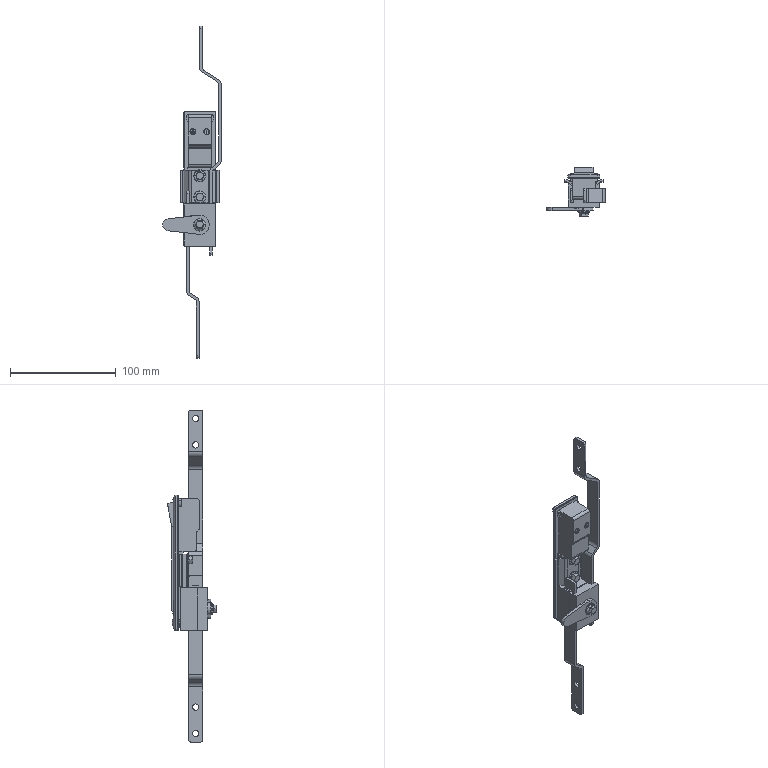Part | SolidWorks | 1 solid | 496 faces | box 55.3 x 46.477 x 314 mm | volume 91025 mm3 | plane 264 | cylinder 185 | spline 32 | cone 15 | commonest cylinder face diameters 1 x38 16 x26 1.6 x24 4 x24 10 x12 2 x10